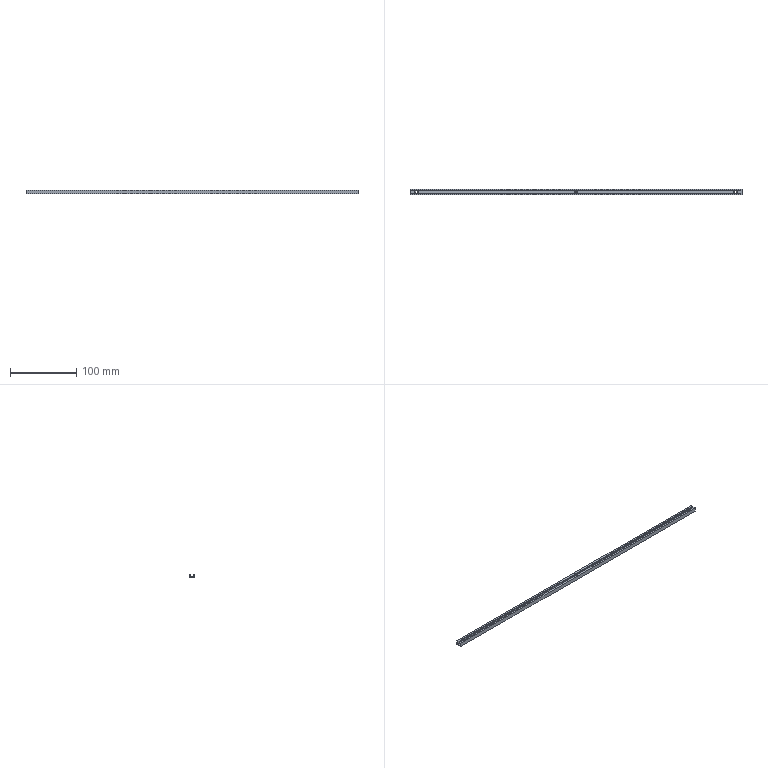Part | STEP file | 001-008-SENAM33H-500-V10-W250-X490 | 1 solid | 56 faces | box 500 x 9 x 6 mm | volume 15737 mm3 | plane 44 | cylinder 6 | cone 6 | commonest cylinder face diameters 6 x6